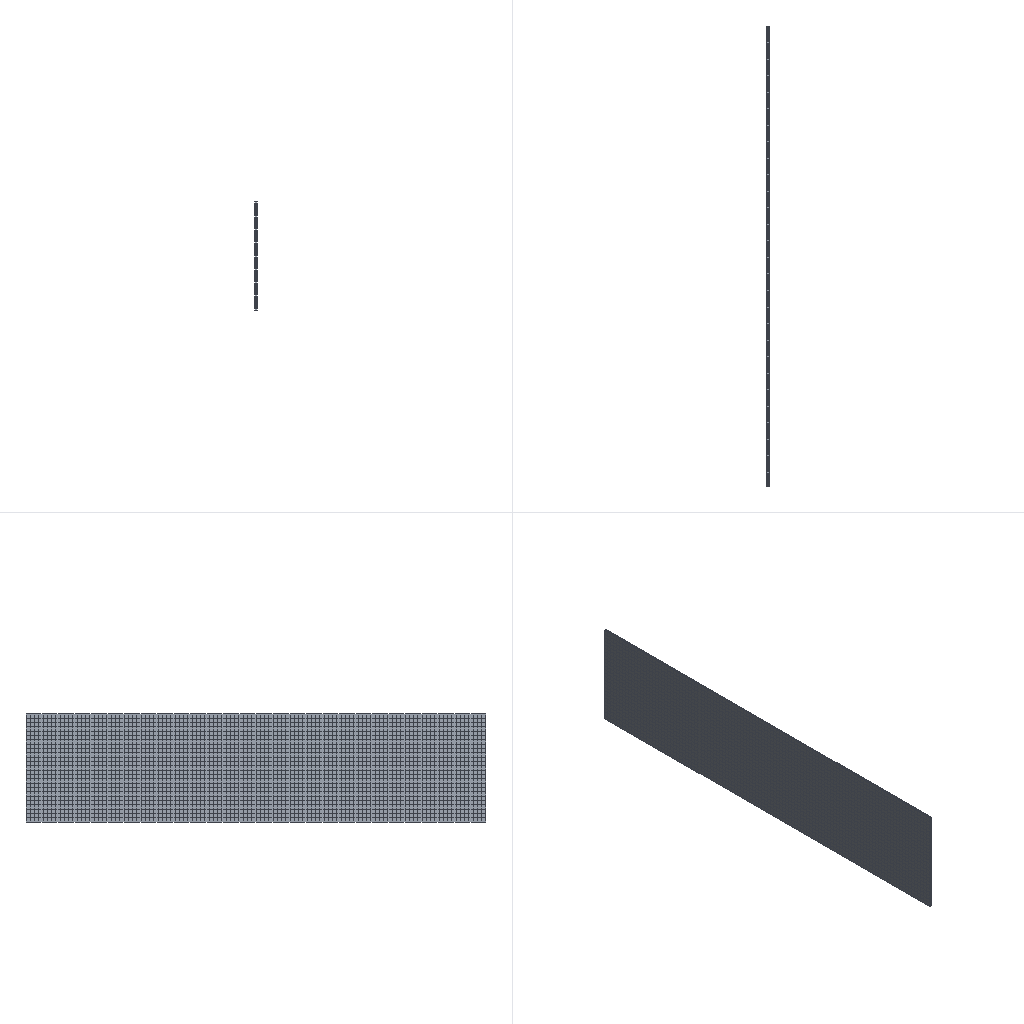Simulation study | abaqus
Set-up summary:
category,name,step,type,value,unit,region
solver,abaqus
solver,version,,,Abaqus/Explicit 2020
units,not stated in the deck,,not stated
analysis,deck,,transient,transient
load_step,Step-1,Step-1,transient
load_step,requested,,,1
mesh,nodes,,,32660
mesh,elements,,,33270
element_type,R3D3,,rigid,8232
element_type,R3D4,,rigid,11538
element_type,C3D8R,,solid,13500
load,load commands in deck,,count,4
bc,support commands in deck,,count,13
material,MATERIAL-1,,in results
check,setup vs results,,match,"per instance, exact: element labels, types and connectivity; labels of the nodes the elements use; coordinates of those nodes at SINGLE_PRECISION in 3 of 3 instance(s)"
Abaqus input file, long lists of numbers shortened:
*Heading
** Job name: Job-1 Model name: Model-1
** Generated by: Abaqus/CAE 2020
*Preprint, echo=NO, model=NO, history=NO, contact=NO
**
** PARTS
**
*Part, name=work-1
*Node
      1,   720.09,   -2609.6,   33.02
      2,    719.582,   -2609.6,   33.02
** (17002 more lines like these left out)
*Element, type=C3D8R
    1,   655,   656,   662,   661,     1,     2,     8,     7
    2,   656,   657,   663,   662,     2,     3,     9,     8
** (13498 more lines like these left out)
*Nset, nset=Set-2, generate
     1,  17004,      1
*Elset, elset=Set-2, generate
     1,  13500,      1
** Section: Section-1
*Solid Section, elset=Set-2, material=Material-1
,
*End Part
**
*Part, name=work-2
*Node
      1,   2138.247,   232.468,  -10.16
      2,   2144.895,   228.744,  -10.16
** (7799 more lines like these left out)
*Element, type=R3D4
1, 1, 2, 3, 4
2, 5, 6, 3, 2
** (5725 more lines like these left out)
*Element, type=R3D3
1621, 4, 6, 7
1622, 3, 6, 4
** (4146 more lines like these left out)
*Node
   7802,    1437.639,   0.1377,  -93.98
*Nset, nset=work-2-RefPt_, internal
7802,
*Elset, elset=work-2, generate
    1,  9875,     1
*End Part
**
*Part, name=work-3
*Node
      1,  -727.033,  -127.491,   -10.16
      2,  -733.066,   -122.836,   4.572
** (7851 more lines like these left out)
*Element, type=R3D4
1, 1, 2, 3, 4
2, 5, 6, 3, 2
** (5809 more lines like these left out)
*Element, type=R3D3
1625, 6, 7, 3
1626, 3, 7, 4
** (4082 more lines like these left out)
*Node
   7854, -0.001989, 1.92329708e-10,  -93.98
*Nset, nset=work-3-RefPt_, internal
7854,
*Elset, elset=work-3, generate
    1,  9895,     1
*End Part
**
**
** ASSEMBLY
**
*Assembly, name=Assembly
**
*Instance, name=work-1-1, part=work-1
          0.,        2400.,           0.
*End Instance
**
*Instance, name=work-2-1, part=work-2
*End Instance
**
*Instance, name=work-3-1, part=work-3
*End Instance
**
*Nset, nset=Set-1, instance=work-1-1
     1,     2,     3,     4,     5,     6,     7,     8,     9,    10,    11,    12,    13,    14,    15,    16
    17,    18,    19,    20,    21,    22,    23,    24,    25,    26,    27,    28,    29,    30,    31,    32
** (80 more lines like these left out)
*Elset, elset=Set-1, instance=work-1-1
     1,     2,     3,     4,     5,     6,     7,     8,     9,    10,    11,    12,    13,    14,    15,    16
    17,    18,    19,    20,    21,    22,    23,    24,    25,    26,    27,    28,    29,    30,    31,    32
** (66 more lines like these left out)
*Nset, nset=Set-2, instance=work-2-1
 7802,
*Nset, nset=Set-3, instance=work-3-1
 7854,
*Rigid Body, ref node=work-2-1.work-2-RefPt_, elset=work-2-1.work-2
*Rigid Body, ref node=work-3-1.work-3-RefPt_, elset=work-3-1.work-3
*End Assembly
**
** MATERIALS
**
*Material, name=Material-1
*Density
 2.7e-09,
*Elastic
72000., 0.29
**
** INTERACTION PROPERTIES
**
*Surface Interaction, name=IntProp-1
*Friction
 0.1,
*Surface Behavior, pressure-overclosure=HARD
** ----------------------------------------------------------------
**
** STEP: Step-1
**
*Step, name=Step-1, nlgeom=YES
*Dynamic, Explicit
, 0.032
*Bulk Viscosity
0.06, 1.2
** Mass Scaling: Semi-Automatic
**               Whole Model
*Fixed Mass Scaling, factor=500.
**
** BOUNDARY CONDITIONS
**
** Name: BC-1 Type: 位移/转角
*Boundary
Set-1, 3, 3
** Name: BC-2 Type: 速度/角速度
*Boundary, type=VELOCITY
Set-2, 1, 1
Set-2, 2, 2, -1000.
Set-2, 3, 3
Set-2, 4, 4
Set-2, 5, 5
Set-2, 6, 6, -31.4
** Name: BC-2-Copy Type: 速度/角速度
*Boundary, type=VELOCITY
Set-3, 1, 1
Set-3, 2, 2, -1000.
Set-3, 3, 3
Set-3, 4, 4
Set-3, 5, 5
Set-3, 6, 6, 31.4
**
** INTERACTIONS
**
** Interaction: Int-1
*Contact, op=NEW
*Contact Inclusions, ALL EXTERIOR
*Contact Property Assignment
 ,  , IntProp-1
**
** OUTPUT REQUESTS
**
*Restart, write, number interval=1, time marks=NO
**
** FIELD OUTPUT: F-Output-1
**
*Output, field, number interval=50
*Node Output
A, CF, RF, RM, RT, U, V
*Element Output, directions=YES
E, EVF, LE, MISES, MISESMAX, MISESONLY, PE, PEEQ, PEEQMAX, PEEQT, PEEQVAVG, PEMAG, PEVAVG, PRESSONLY, S, SF
SSAVG, SVAVG, VEEQ, YIELDPOT
*Contact Output
CDISP, CSTRESS
**
** HISTORY OUTPUT: H-Output-1
**
*Output, history, variable=PRESELECT
*End Step
Results summary:
result,step,Step-1,completed,increments=20568 time=0.032/0.032
result,analysis,,,transient
result,last_loadstep,,,1
result,primary field,,,U
result,reaction total,,FX,-149537.0,model units
result,reaction total,,FY,677398.0,model units
result,reaction total,,FZ,345440.654,model units